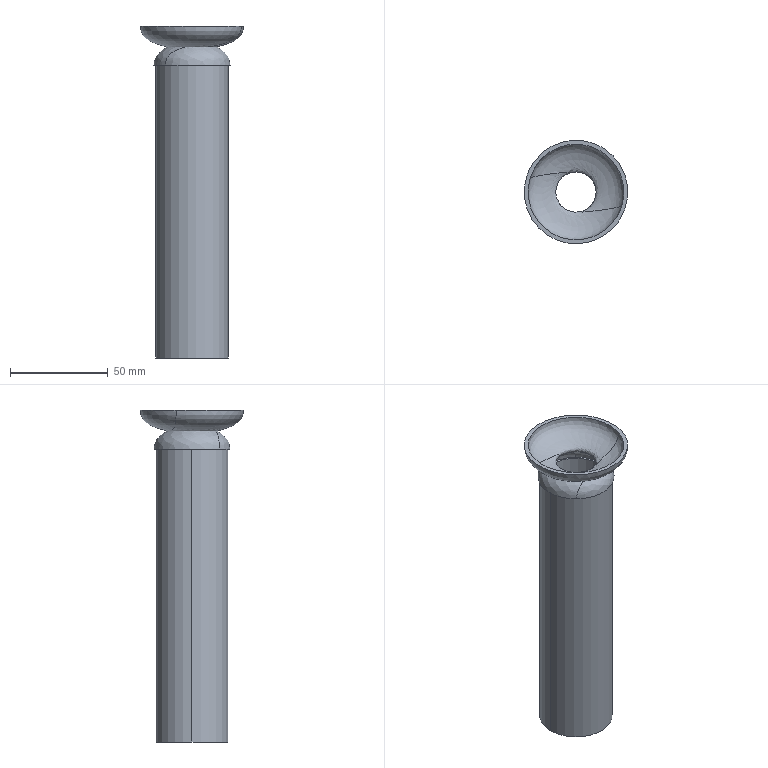Part | SolidWorks | features Blend 1, ExtruThin 1 | 1 solid | 14 faces | box 53.043 x 53.043 x 170 mm | volume 40176 mm3 | spline 6 | cylinder 4 | plane 4 | commonest cylinder face diameters 33 x2 37 x2